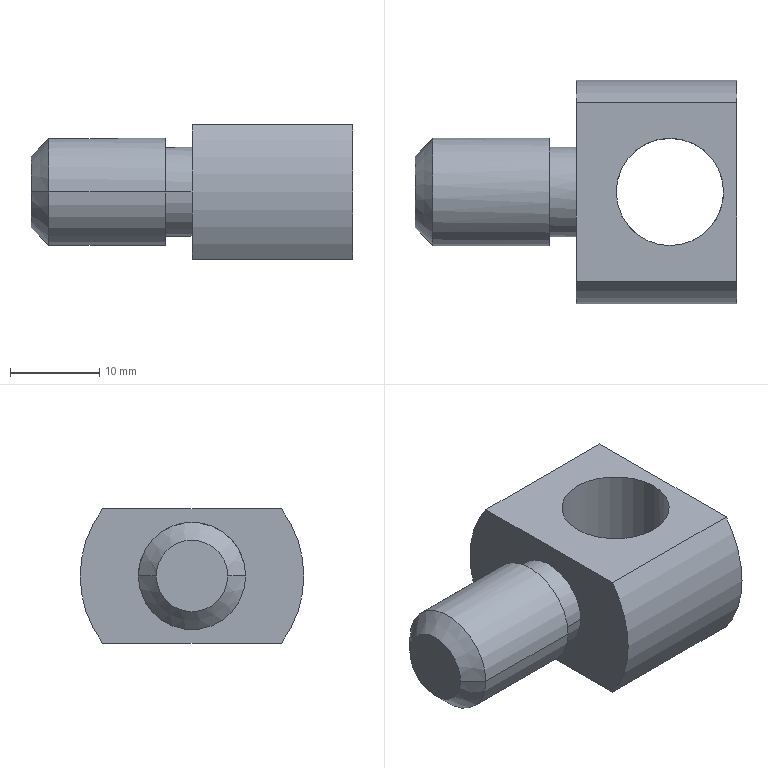Part | STEP file | Positioning_id2194_x_t | 1 solid | 16 faces | box 36 x 25 x 15 mm | volume 6488 mm3 | cylinder 8 | plane 6 | cone 2 | commonest cylinder face diameters 12 x4 10 x2 25 x2
STEP:
#1=CARTESIAN_POINT('',(0.,0.,0.));
#2=DIRECTION('',(0.,0.,1.));
#3=DIRECTION('',(1.,0.,0.));
#4=AXIS2_PLACEMENT_3D('',#1,#2,#3);
#5=CARTESIAN_POINT('',(-1029.002,410.,41.));
#6=VERTEX_POINT('',#5);
#7=CARTESIAN_POINT('',(-1031.002,412.,41.));
#8=VERTEX_POINT('',#7);
#9=CARTESIAN_POINT('',(-1031.002,412.,41.));
#10=DIRECTION('',(-0.7071,0.7071,0.));
#11=VECTOR('',#10,1.);
#12=LINE('',#9,#11);
#13=CARTESIAN_POINT('',(-1029.002,416.,41.));
#14=DIRECTION('',(1.,0.,0.));
#15=DIRECTION('',(0.,-1.,0.));
#16=AXIS2_PLACEMENT_3D('',#13,#14,#15);
#17=CONICAL_SURFACE('',#16,6.,0.7854);
#18=CARTESIAN_POINT('',(0.,-2.));
#19=DIRECTION('',(0.,-1.));
#20=VECTOR('',#19,1.);
#21=LINE('',#18,#20);
#22=(GEOMETRIC_REPRESENTATION_CONTEXT(2)PARAMETRIC_REPRESENTATION_CONTEXT()REPRESENTATION_CONTEXT('',''));
#23=DEFINITIONAL_REPRESENTATION('',(#21),#22);
#24=PCURVE('',#17,#23);
#25=CARTESIAN_POINT('',(-1029.002,416.,41.));
#26=DIRECTION('',(1.,0.,0.));
#27=DIRECTION('',(0.,-1.,0.));
#28=AXIS2_PLACEMENT_3D('',#25,#26,#27);
#29=CONICAL_SURFACE('',#28,6.,0.7854);
#30=CARTESIAN_POINT('',(6.283,-2.));
#31=DIRECTION('',(0.,-1.));
#32=VECTOR('',#31,1.);
#33=LINE('',#30,#32);
#34=(GEOMETRIC_REPRESENTATION_CONTEXT(2)PARAMETRIC_REPRESENTATION_CONTEXT()REPRESENTATION_CONTEXT('',''));
#35=DEFINITIONAL_REPRESENTATION('',(#33),#34);
#36=PCURVE('',#29,#35);
#37=SURFACE_CURVE('',#12,(#24,#36),.PCURVE_S1.);
#38=EDGE_CURVE('',#6,#8,#37,.T.);
#39=ORIENTED_EDGE('',*,*,#38,.T.);
#40=CARTESIAN_POINT('',(-1031.002,420.,41.));
#41=VERTEX_POINT('',#40);
#42=CARTESIAN_POINT('',(-1031.002,416.,41.));
#43=DIRECTION('',(-1.,0.,0.));
#44=DIRECTION('',(0.,1.,0.));
#45=AXIS2_PLACEMENT_3D('',#42,#43,#44);
#46=CIRCLE('',#45,4.);
#47=CARTESIAN_POINT('',(3.142,-2.));
#48=DIRECTION('',(-1.,0.));
#49=VECTOR('',#48,1.);
#50=LINE('',#47,#49);
#51=(GEOMETRIC_REPRESENTATION_CONTEXT(2)PARAMETRIC_REPRESENTATION_CONTEXT()REPRESENTATION_CONTEXT('',''));
#52=DEFINITIONAL_REPRESENTATION('',(#50),#51);
#53=PCURVE('',#17,#52);
#54=CARTESIAN_POINT('',(-1031.002,416.,41.));
#55=DIRECTION('',(-1.,0.,0.));
#56=DIRECTION('',(0.,1.,0.));
#57=AXIS2_PLACEMENT_3D('',#54,#55,#56);
#58=PLANE('',#57);
#59=CARTESIAN_POINT('',(0.,0.));
#60=DIRECTION('',(1.,0.));
#61=AXIS2_PLACEMENT_2D('',#59,#60);
#62=CIRCLE('',#61,4.);
#63=(GEOMETRIC_REPRESENTATION_CONTEXT(2)PARAMETRIC_REPRESENTATION_CONTEXT()REPRESENTATION_CONTEXT('',''));
#64=DEFINITIONAL_REPRESENTATION('',(#62),#63);
#65=PCURVE('',#58,#64);
#66=SURFACE_CURVE('',#46,(#53,#65),.PCURVE_S1.);
#67=EDGE_CURVE('',#41,#8,#66,.T.);
#68=ORIENTED_EDGE('',*,*,#67,.F.);
#69=CARTESIAN_POINT('',(-1029.002,422.,41.));
#70=VERTEX_POINT('',#69);
#71=CARTESIAN_POINT('',(-1031.002,420.,41.));
#72=DIRECTION('',(0.7071,0.7071,0.));
#73=VECTOR('',#72,1.);
#74=LINE('',#71,#73);
#75=CARTESIAN_POINT('',(3.142,-2.));
#76=DIRECTION('',(0.,1.));
#77=VECTOR('',#76,1.);
#78=LINE('',#75,#77);
#79=(GEOMETRIC_REPRESENTATION_CONTEXT(2)PARAMETRIC_REPRESENTATION_CONTEXT()REPRESENTATION_CONTEXT('',''));
#80=DEFINITIONAL_REPRESENTATION('',(#78),#79);
#81=PCURVE('',#17,#80);
#82=CARTESIAN_POINT('',(3.142,-2.));
#83=DIRECTION('',(0.,1.));
#84=VECTOR('',#83,1.);
#85=LINE('',#82,#84);
#86=(GEOMETRIC_REPRESENTATION_CONTEXT(2)PARAMETRIC_REPRESENTATION_CONTEXT()REPRESENTATION_CONTEXT('',''));
#87=DEFINITIONAL_REPRESENTATION('',(#85),#86);
#88=PCURVE('',#29,#87);
#89=SURFACE_CURVE('',#74,(#81,#88),.PCURVE_S1.);
#90=EDGE_CURVE('',#41,#70,#89,.T.);
#91=ORIENTED_EDGE('',*,*,#90,.T.);
#92=CARTESIAN_POINT('',(-1029.002,416.,41.));
#93=DIRECTION('',(1.,0.,0.));
#94=DIRECTION('',(0.,-1.,0.));
#95=AXIS2_PLACEMENT_3D('',#92,#93,#94);
#96=CIRCLE('',#95,6.);
#97=CARTESIAN_POINT('',(0.,0.));
#98=DIRECTION('',(1.,0.));
#99=VECTOR('',#98,1.);
#100=LINE('',#97,#99);
#101=(GEOMETRIC_REPRESENTATION_CONTEXT(2)PARAMETRIC_REPRESENTATION_CONTEXT()REPRESENTATION_CONTEXT('',''));
#102=DEFINITIONAL_REPRESENTATION('',(#100),#101);
#103=PCURVE('',#17,#102);
#104=CARTESIAN_POINT('',(-1016.002,416.,41.));
#105=DIRECTION('',(1.,0.,0.));
#106=DIRECTION('',(0.,1.,0.));
#107=AXIS2_PLACEMENT_3D('',#104,#105,#106);
#108=CYLINDRICAL_SURFACE('',#107,6.);
#109=CARTESIAN_POINT('',(3.142,-13.));
#110=DIRECTION('',(1.,0.));
#111=VECTOR('',#110,1.);
#112=LINE('',#109,#111);
#113=(GEOMETRIC_REPRESENTATION_CONTEXT(2)PARAMETRIC_REPRESENTATION_CONTEXT()REPRESENTATION_CONTEXT('',''));
#114=DEFINITIONAL_REPRESENTATION('',(#112),#113);
#115=PCURVE('',#108,#114);
#116=SURFACE_CURVE('',#96,(#103,#115),.PCURVE_S1.);
#117=EDGE_CURVE('',#6,#70,#116,.T.);
#118=ORIENTED_EDGE('',*,*,#117,.F.);
#119=EDGE_LOOP('',(#39,#68,#91,#118));
#120=FACE_BOUND('',#119,.T.);
#121=ADVANCED_FACE('',(#120),#17,.T.);
#122=CARTESIAN_POINT('',(-1016.002,422.,41.));
#123=VERTEX_POINT('',#122);
#124=CARTESIAN_POINT('',(-1016.002,422.,41.));
#125=DIRECTION('',(1.,0.,0.));
#126=VECTOR('',#125,1.);
#127=LINE('',#124,#126);
#128=CARTESIAN_POINT('',(6.283,0.));
#129=DIRECTION('',(0.,1.));
#130=VECTOR('',#129,1.);
#131=LINE('',#128,#130);
#132=(GEOMETRIC_REPRESENTATION_CONTEXT(2)PARAMETRIC_REPRESENTATION_CONTEXT()REPRESENTATION_CONTEXT('',''));
#133=DEFINITIONAL_REPRESENTATION('',(#131),#132);
#134=PCURVE('',#108,#133);
#135=CARTESIAN_POINT('',(-1016.002,416.,41.));
#136=DIRECTION('',(1.,0.,0.));
#137=DIRECTION('',(0.,1.,0.));
#138=AXIS2_PLACEMENT_3D('',#135,#136,#137);
#139=CYLINDRICAL_SURFACE('',#138,6.);
#140=CARTESIAN_POINT('',(0.,0.));
#141=DIRECTION('',(0.,1.));
#142=VECTOR('',#141,1.);
#143=LINE('',#140,#142);
#144=(GEOMETRIC_REPRESENTATION_CONTEXT(2)PARAMETRIC_REPRESENTATION_CONTEXT()REPRESENTATION_CONTEXT('',''));
#145=DEFINITIONAL_REPRESENTATION('',(#143),#144);
#146=PCURVE('',#139,#145);
#147=SURFACE_CURVE('',#127,(#134,#146),.PCURVE_S1.);
#148=EDGE_CURVE('',#70,#123,#147,.T.);
#149=ORIENTED_EDGE('',*,*,#148,.T.);
#150=CARTESIAN_POINT('',(-1016.002,410.,41.));
#151=VERTEX_POINT('',#150);
#152=CARTESIAN_POINT('',(-1016.002,416.,41.));
#153=DIRECTION('',(-1.,0.,0.));
#154=DIRECTION('',(0.,1.,0.));
#155=AXIS2_PLACEMENT_3D('',#152,#153,#154);
#156=CIRCLE('',#155,6.);
#157=CARTESIAN_POINT('',(6.283,0.));
#158=DIRECTION('',(-1.,0.));
#159=VECTOR('',#158,1.);
#160=LINE('',#157,#159);
#161=(GEOMETRIC_REPRESENTATION_CONTEXT(2)PARAMETRIC_REPRESENTATION_CONTEXT()REPRESENTATION_CONTEXT('',''));
#162=DEFINITIONAL_REPRESENTATION('',(#160),#161);
#163=PCURVE('',#108,#162);
#164=CARTESIAN_POINT('',(-1016.002,416.,41.));
#165=DIRECTION('',(1.,0.,0.));
#166=DIRECTION('',(0.,-1.,0.));
#167=AXIS2_PLACEMENT_3D('',#164,#165,#166);
#168=PLANE('',#167);
#169=CARTESIAN_POINT('',(-6.,0.));
#170=CARTESIAN_POINT('',(-6.,10.392));
#171=CARTESIAN_POINT('',(3.,5.196));
#172=CARTESIAN_POINT('',(12.,0.));
#173=CARTESIAN_POINT('',(3.,-5.196));
#174=CARTESIAN_POINT('',(-6.,-10.392));
#175=CARTESIAN_POINT('',(-6.,0.));
#176=(BOUNDED_CURVE()B_SPLINE_CURVE(2,(#169,#170,#171,#172,#173,#174,#175),.UNSPECIFIED.,.T.,.F.)B_SPLINE_CURVE_WITH_KNOTS((1,2,2,2,2,1),(-2.094,0.,2.094,4.189,6.283,8.378),.UNSPECIFIED.)CURVE()GEOMETRIC_REPRESENTATION_ITEM()RATIONAL_B_SPLINE_CURVE((1.,0.5,1.,0.5,1.,0.5,1.))REPRESENTATION_ITEM(''));
#177=(GEOMETRIC_REPRESENTATION_CONTEXT(2)PARAMETRIC_REPRESENTATION_CONTEXT()REPRESENTATION_CONTEXT('',''));
#178=DEFINITIONAL_REPRESENTATION('',(#176),#177);
#179=PCURVE('',#168,#178);
#180=SURFACE_CURVE('',#156,(#163,#179),.PCURVE_S1.);
#181=EDGE_CURVE('',#123,#151,#180,.T.);
#182=ORIENTED_EDGE('',*,*,#181,.T.);
#183=CARTESIAN_POINT('',(-1016.002,410.,41.));
#184=DIRECTION('',(-1.,0.,0.));
#185=VECTOR('',#184,1.);
#186=LINE('',#183,#185);
#187=CARTESIAN_POINT('',(3.142,0.));
#188=DIRECTION('',(0.,-1.));
#189=VECTOR('',#188,1.);
#190=LINE('',#187,#189);
#191=(GEOMETRIC_REPRESENTATION_CONTEXT(2)PARAMETRIC_REPRESENTATION_CONTEXT()REPRESENTATION_CONTEXT('',''));
#192=DEFINITIONAL_REPRESENTATION('',(#190),#191);
#193=PCURVE('',#108,#192);
#194=CARTESIAN_POINT('',(3.142,0.));
#195=DIRECTION('',(0.,-1.));
#196=VECTOR('',#195,1.);
#197=LINE('',#194,#196);
#198=(GEOMETRIC_REPRESENTATION_CONTEXT(2)PARAMETRIC_REPRESENTATION_CONTEXT()REPRESENTATION_CONTEXT('',''));
#199=DEFINITIONAL_REPRESENTATION('',(#197),#198);
#200=PCURVE('',#139,#199);
#201=SURFACE_CURVE('',#186,(#193,#200),.PCURVE_S1.);
#202=EDGE_CURVE('',#151,#6,#201,.T.);
#203=ORIENTED_EDGE('',*,*,#202,.T.);
#204=ORIENTED_EDGE('',*,*,#117,.T.);
#205=EDGE_LOOP('',(#149,#182,#203,#204));
#206=FACE_BOUND('',#205,.T.);
#207=ADVANCED_FACE('',(#206),#108,.T.);
#208=CARTESIAN_POINT('',(-1016.002,411.,41.));
#209=VERTEX_POINT('',#208);
#210=CARTESIAN_POINT('',(-1016.002,421.,41.));
#211=VERTEX_POINT('',#210);
#212=CARTESIAN_POINT('',(-1016.002,416.,41.));
#213=DIRECTION('',(-1.,0.,0.));
#214=DIRECTION('',(0.,-1.,0.));
#215=AXIS2_PLACEMENT_3D('',#212,#213,#214);
#216=CIRCLE('',#215,5.);
#217=CARTESIAN_POINT('',(5.,0.));
#218=CARTESIAN_POINT('',(5.,-8.66));
#219=CARTESIAN_POINT('',(-2.5,-4.33));
#220=CARTESIAN_POINT('',(-10.,0.));
#221=CARTESIAN_POINT('',(-2.5,4.33));
#222=CARTESIAN_POINT('',(5.,8.66));
#223=CARTESIAN_POINT('',(5.,0.));
#224=(BOUNDED_CURVE()B_SPLINE_CURVE(2,(#217,#218,#219,#220,#221,#222,#223),.UNSPECIFIED.,.T.,.F.)B_SPLINE_CURVE_WITH_KNOTS((1,2,2,2,2,1),(-2.094,0.,2.094,4.189,6.283,8.378),.UNSPECIFIED.)CURVE()GEOMETRIC_REPRESENTATION_ITEM()RATIONAL_B_SPLINE_CURVE((1.,0.5,1.,0.5,1.,0.5,1.))REPRESENTATION_ITEM(''));
#225=(GEOMETRIC_REPRESENTATION_CONTEXT(2)PARAMETRIC_REPRESENTATION_CONTEXT()REPRESENTATION_CONTEXT('',''));
#226=DEFINITIONAL_REPRESENTATION('',(#224),#225);
#227=PCURVE('',#168,#226);
#228=CARTESIAN_POINT('',(-1013.002,416.,41.));
#229=DIRECTION('',(1.,0.,0.));
#230=DIRECTION('',(0.,1.,0.));
#231=AXIS2_PLACEMENT_3D('',#228,#229,#230);
#232=CYLINDRICAL_SURFACE('',#231,5.);
#233=CARTESIAN_POINT('',(3.142,-3.));
#234=DIRECTION('',(-1.,0.));
#235=VECTOR('',#234,1.);
#236=LINE('',#233,#235);
#237=(GEOMETRIC_REPRESENTATION_CONTEXT(2)PARAMETRIC_REPRESENTATION_CONTEXT()REPRESENTATION_CONTEXT('',''));
#238=DEFINITIONAL_REPRESENTATION('',(#236),#237);
#239=PCURVE('',#232,#238);
#240=SURFACE_CURVE('',#216,(#227,#239),.PCURVE_S1.);
#241=EDGE_CURVE('',#209,#211,#240,.T.);
#242=ORIENTED_EDGE('',*,*,#241,.T.);
#243=CARTESIAN_POINT('',(-1016.002,416.,41.));
#244=DIRECTION('',(-1.,0.,0.));
#245=DIRECTION('',(0.,1.,0.));
#246=AXIS2_PLACEMENT_3D('',#243,#244,#245);
#247=CIRCLE('',#246,5.);
#248=CARTESIAN_POINT('',(-5.,0.));
#249=CARTESIAN_POINT('',(-5.,8.66));
#250=CARTESIAN_POINT('',(2.5,4.33));
#251=CARTESIAN_POINT('',(10.,0.));
#252=CARTESIAN_POINT('',(2.5,-4.33));
#253=CARTESIAN_POINT('',(-5.,-8.66));
#254=CARTESIAN_POINT('',(-5.,0.));
#255=(BOUNDED_CURVE()B_SPLINE_CURVE(2,(#248,#249,#250,#251,#252,#253,#254),.UNSPECIFIED.,.T.,.F.)B_SPLINE_CURVE_WITH_KNOTS((1,2,2,2,2,1),(-2.094,0.,2.094,4.189,6.283,8.378),.UNSPECIFIED.)CURVE()GEOMETRIC_REPRESENTATION_ITEM()RATIONAL_B_SPLINE_CURVE((1.,0.5,1.,0.5,1.,0.5,1.))REPRESENTATION_ITEM(''));
#256=(GEOMETRIC_REPRESENTATION_CONTEXT(2)PARAMETRIC_REPRESENTATION_CONTEXT()REPRESENTATION_CONTEXT('',''));
#257=DEFINITIONAL_REPRESENTATION('',(#255),#256);
#258=PCURVE('',#168,#257);
#259=CARTESIAN_POINT('',(-1013.002,416.,41.));
#260=DIRECTION('',(1.,0.,0.));
#261=DIRECTION('',(0.,1.,0.));
#262=AXIS2_PLACEMENT_3D('',#259,#260,#261);
#263=CYLINDRICAL_SURFACE('',#262,5.);
#264=CARTESIAN_POINT('',(6.283,-3.));
#265=DIRECTION('',(-1.,0.));
#266=VECTOR('',#265,1.);
#267=LINE('',#264,#266);
#268=(GEOMETRIC_REPRESENTATION_CONTEXT(2)PARAMETRIC_REPRESENTATION_CONTEXT()REPRESENTATION_CONTEXT('',''));
#269=DEFINITIONAL_REPRESENTATION('',(#267),#268);
#270=PCURVE('',#263,#269);
#271=SURFACE_CURVE('',#247,(#258,#270),.PCURVE_S1.);
#272=EDGE_CURVE('',#211,#209,#271,.T.);
#273=ORIENTED_EDGE('',*,*,#272,.T.);
#274=EDGE_LOOP('',(#242,#273));
#275=FACE_BOUND('',#274,.T.);
#276=CARTESIAN_POINT('',(-1016.002,410.,41.));
#277=CARTESIAN_POINT('',(-1016.002,410.,47.));
#278=CARTESIAN_POINT('',(-1016.002,416.,50.));
#279=CARTESIAN_POINT('',(-1016.002,422.,47.));
#280=CARTESIAN_POINT('',(-1016.002,422.,41.));
#281=(BOUNDED_CURVE()B_SPLINE_CURVE(4,(#276,#277,#278,#279,#280),.UNSPECIFIED.,.F.,.F.)B_SPLINE_CURVE_WITH_KNOTS((5,5),(0.,1.),.PIECEWISE_BEZIER_KNOTS.)CURVE()GEOMETRIC_REPRESENTATION_ITEM()RATIONAL_B_SPLINE_CURVE((1.,0.7071,0.6667,0.7071,1.))REPRESENTATION_ITEM(''));
#282=CARTESIAN_POINT('',(6.,0.));
#283=CARTESIAN_POINT('',(6.,-6.));
#284=CARTESIAN_POINT('',(0.,-9.));
#285=CARTESIAN_POINT('',(-6.,-6.));
#286=CARTESIAN_POINT('',(-6.,0.));
#287=(BOUNDED_CURVE()B_SPLINE_CURVE(4,(#282,#283,#284,#285,#286),.UNSPECIFIED.,.F.,.F.)B_SPLINE_CURVE_WITH_KNOTS((5,5),(0.,1.),.PIECEWISE_BEZIER_KNOTS.)CURVE()GEOMETRIC_REPRESENTATION_ITEM()RATIONAL_B_SPLINE_CURVE((1.,0.7071,0.6667,0.7071,1.))REPRESENTATION_ITEM(''));
#288=(GEOMETRIC_REPRESENTATION_CONTEXT(2)PARAMETRIC_REPRESENTATION_CONTEXT()REPRESENTATION_CONTEXT('',''));
#289=DEFINITIONAL_REPRESENTATION('',(#287),#288);
#290=PCURVE('',#168,#289);
#291=CARTESIAN_POINT('',(3.142,0.));
#292=CARTESIAN_POINT('',(3.099,0.));
#293=CARTESIAN_POINT('',(3.012,0.));
#294=CARTESIAN_POINT('',(2.878,0.));
#295=CARTESIAN_POINT('',(2.742,0.));
#296=CARTESIAN_POINT('',(2.602,0.));
#297=CARTESIAN_POINT('',(2.46,0.));
#298=CARTESIAN_POINT('',(2.316,0.));
#299=CARTESIAN_POINT('',(2.169,0.));
#300=CARTESIAN_POINT('',(2.021,0.));
#301=CARTESIAN_POINT('',(1.872,0.));
#302=CARTESIAN_POINT('',(1.721,0.));
#303=CARTESIAN_POINT('',(1.571,0.));
#304=CARTESIAN_POINT('',(1.42,0.));
#305=CARTESIAN_POINT('',(1.27,0.));
#306=CARTESIAN_POINT('',(1.121,0.));
#307=CARTESIAN_POINT('',(0.9725,0.));
#308=CARTESIAN_POINT('',(0.8261,0.));
#309=CARTESIAN_POINT('',(0.6816,0.));
#310=CARTESIAN_POINT('',(0.5394,0.));
#311=CARTESIAN_POINT('',(0.3999,0.));
#312=CARTESIAN_POINT('',(0.2633,0.));
#313=CARTESIAN_POINT('',(0.1297,0.));
#314=CARTESIAN_POINT('',(0.04285,0.));
#315=CARTESIAN_POINT('',(0.,0.));
#316=B_SPLINE_CURVE_WITH_KNOTS('',3,(#291,#292,#293,#294,#295,#296,#297,#298,#299,#300,#301,#302,#303,#304,#305,#306,#307,#308,#309,#310,#311,#312,#313,#314,#315),.UNSPECIFIED.,.F.,.F.,(4,1,1,1,1,1,1,1,1,1,1,1,1,1,1,1,1,1,1,1,1,1,4),(0.,0.04545,0.09091,0.1364,0.1818,0.2273,0.2727,0.3182,0.3636,0.4091,0.4545,0.5,0.5455,0.5909,0.6364,0.6818,0.7273,0.7727,0.8182,0.8636,0.9091,0.9545,1.),.QUASI_UNIFORM_KNOTS.);
#317=(GEOMETRIC_REPRESENTATION_CONTEXT(2)PARAMETRIC_REPRESENTATION_CONTEXT()REPRESENTATION_CONTEXT('',''));
#318=DEFINITIONAL_REPRESENTATION('',(#316),#317);
#319=PCURVE('',#139,#318);
#320=SURFACE_CURVE('',#281,(#290,#319),.PCURVE_S1.);
#321=EDGE_CURVE('',#151,#123,#320,.T.);
#322=ORIENTED_EDGE('',*,*,#321,.F.);
#323=ORIENTED_EDGE('',*,*,#181,.F.);
#324=EDGE_LOOP('',(#322,#323));
#325=FACE_BOUND('',#324,.T.);
#326=ADVANCED_FACE('',(#275,#325),#168,.T.);
#327=ORIENTED_EDGE('',*,*,#67,.T.);
#328=CARTESIAN_POINT('',(-1031.002,412.,41.));
#329=CARTESIAN_POINT('',(-1031.002,412.,45.));
#330=CARTESIAN_POINT('',(-1031.002,416.,47.));
#331=CARTESIAN_POINT('',(-1031.002,420.,45.));
#332=CARTESIAN_POINT('',(-1031.002,420.,41.));
#333=(BOUNDED_CURVE()B_SPLINE_CURVE(4,(#328,#329,#330,#331,#332),.UNSPECIFIED.,.F.,.F.)B_SPLINE_CURVE_WITH_KNOTS((5,5),(0.,1.),.PIECEWISE_BEZIER_KNOTS.)CURVE()GEOMETRIC_REPRESENTATION_ITEM()RATIONAL_B_SPLINE_CURVE((1.,0.7071,0.6667,0.7071,1.))REPRESENTATION_ITEM(''));
#334=CARTESIAN_POINT('',(-4.,0.));
#335=CARTESIAN_POINT('',(-4.,-4.));
#336=CARTESIAN_POINT('',(0.,-6.));
#337=CARTESIAN_POINT('',(4.,-4.));
#338=CARTESIAN_POINT('',(4.,0.));
#339=(BOUNDED_CURVE()B_SPLINE_CURVE(4,(#334,#335,#336,#337,#338),.UNSPECIFIED.,.F.,.F.)B_SPLINE_CURVE_WITH_KNOTS((5,5),(0.,1.),.PIECEWISE_BEZIER_KNOTS.)CURVE()GEOMETRIC_REPRESENTATION_ITEM()RATIONAL_B_SPLINE_CURVE((1.,0.7071,0.6667,0.7071,1.))REPRESENTATION_ITEM(''));
#340=(GEOMETRIC_REPRESENTATION_CONTEXT(2)PARAMETRIC_REPRESENTATION_CONTEXT()REPRESENTATION_CONTEXT('',''));
#341=DEFINITIONAL_REPRESENTATION('',(#339),#340);
#342=PCURVE('',#58,#341);
#343=CARTESIAN_POINT('',(6.283,-2.));
#344=CARTESIAN_POINT('',(6.24,-2.));
#345=CARTESIAN_POINT('',(6.153,-2.));
#346=CARTESIAN_POINT('',(6.02,-2.));
#347=CARTESIAN_POINT('',(5.883,-2.));
#348=CARTESIAN_POINT('',(5.744,-2.));
#349=CARTESIAN_POINT('',(5.602,-2.));
#350=CARTESIAN_POINT('',(5.457,-2.));
#351=CARTESIAN_POINT('',(5.311,-2.));
#352=CARTESIAN_POINT('',(5.163,-2.));
#353=CARTESIAN_POINT('',(5.013,-2.));
#354=CARTESIAN_POINT('',(4.863,-2.));
#355=CARTESIAN_POINT('',(4.712,-2.));
#356=CARTESIAN_POINT('',(4.562,-2.));
#357=CARTESIAN_POINT('',(4.412,-2.));
#358=CARTESIAN_POINT('',(4.262,-2.));
#359=CARTESIAN_POINT('',(4.114,-2.));
#360=CARTESIAN_POINT('',(3.968,-2.));
#361=CARTESIAN_POINT('',(3.823,-2.));
#362=CARTESIAN_POINT('',(3.681,-2.));
#363=CARTESIAN_POINT('',(3.542,-2.));
#364=CARTESIAN_POINT('',(3.405,-2.));
#365=CARTESIAN_POINT('',(3.271,-2.));
#366=CARTESIAN_POINT('',(3.184,-2.));
#367=CARTESIAN_POINT('',(3.142,-2.));
#368=B_SPLINE_CURVE_WITH_KNOTS('',3,(#343,#344,#345,#346,#347,#348,#349,#350,#351,#352,#353,#354,#355,#356,#357,#358,#359,#360,#361,#362,#363,#364,#365,#366,#367),.UNSPECIFIED.,.F.,.F.,(4,1,1,1,1,1,1,1,1,1,1,1,1,1,1,1,1,1,1,1,1,1,4),(0.,0.04545,0.09091,0.1364,0.1818,0.2273,0.2727,0.3182,0.3636,0.4091,0.4545,0.5,0.5455,0.5909,0.6364,0.6818,0.7273,0.7727,0.8182,0.8636,0.9091,0.9545,1.),.QUASI_UNIFORM_KNOTS.);
#369=(GEOMETRIC_REPRESENTATION_CONTEXT(2)PARAMETRIC_REPRESENTATION_CONTEXT()REPRESENTATION_CONTEXT('',''));
#370=DEFINITIONAL_REPRESENTATION('',(#368),#369);
#371=PCURVE('',#29,#370);
#372=SURFACE_CURVE('',#333,(#342,#371),.PCURVE_S1.);
#373=EDGE_CURVE('',#8,#41,#372,.T.);
#374=ORIENTED_EDGE('',*,*,#373,.T.);
#375=EDGE_LOOP('',(#327,#374));
#376=FACE_BOUND('',#375,.T.);
#377=ADVANCED_FACE('',(#376),#58,.T.);
#378=CARTESIAN_POINT('',(-1013.002,421.,41.));
#379=VERTEX_POINT('',#378);
#380=CARTESIAN_POINT('',(-1013.002,421.,41.));
#381=DIRECTION('',(1.,0.,0.));
#382=VECTOR('',#381,1.);
#383=LINE('',#380,#382);
#384=CARTESIAN_POINT('',(6.283,0.));
#385=DIRECTION('',(0.,1.));
#386=VECTOR('',#385,1.);
#387=LINE('',#384,#386);
#388=(GEOMETRIC_REPRESENTATION_CONTEXT(2)PARAMETRIC_REPRESENTATION_CONTEXT()REPRESENTATION_CONTEXT('',''));
#389=DEFINITIONAL_REPRESENTATION('',(#387),#388);
#390=PCURVE('',#263,#389);
#391=CARTESIAN_POINT('',(0.,0.));
#392=DIRECTION('',(0.,1.));
#393=VECTOR('',#392,1.);
#394=LINE('',#391,#393);
#395=(GEOMETRIC_REPRESENTATION_CONTEXT(2)PARAMETRIC_REPRESENTATION_CONTEXT()REPRESENTATION_CONTEXT('',''));
#396=DEFINITIONAL_REPRESENTATION('',(#394),#395);
#397=PCURVE('',#232,#396);
#398=SURFACE_CURVE('',#383,(#390,#397),.PCURVE_S1.);
#399=EDGE_CURVE('',#211,#379,#398,.T.);
#400=ORIENTED_EDGE('',*,*,#399,.T.);
#401=CARTESIAN_POINT('',(-1013.002,411.,41.));
#402=VERTEX_POINT('',#401);
#403=CARTESIAN_POINT('',(-1013.002,416.,41.));
#404=DIRECTION('',(-1.,0.,0.));
#405=DIRECTION('',(0.,1.,0.));
#406=AXIS2_PLACEMENT_3D('',#403,#404,#405);
#407=CIRCLE('',#406,5.);
#408=CARTESIAN_POINT('',(6.283,0.));
#409=DIRECTION('',(-1.,0.));
#410=VECTOR('',#409,1.);
#411=LINE('',#408,#410);
#412=(GEOMETRIC_REPRESENTATION_CONTEXT(2)PARAMETRIC_REPRESENTATION_CONTEXT()REPRESENTATION_CONTEXT('',''));
#413=DEFINITIONAL_REPRESENTATION('',(#411),#412);
#414=PCURVE('',#263,#413);
#415=CARTESIAN_POINT('',(-1013.002,416.,41.));
#416=DIRECTION('',(-1.,0.,0.));
#417=DIRECTION('',(0.,0.,-1.));
#418=AXIS2_PLACEMENT_3D('',#415,#416,#417);
#419=PLANE('',#418);
#420=CARTESIAN_POINT('',(0.,0.));
#421=DIRECTION('',(0.,-1.));
#422=AXIS2_PLACEMENT_2D('',#420,#421);
#423=CIRCLE('',#422,5.);
#424=(GEOMETRIC_REPRESENTATION_CONTEXT(2)PARAMETRIC_REPRESENTATION_CONTEXT()REPRESENTATION_CONTEXT('',''));
#425=DEFINITIONAL_REPRESENTATION('',(#423),#424);
#426=PCURVE('',#419,#425);
#427=SURFACE_CURVE('',#407,(#414,#426),.PCURVE_S1.);
#428=EDGE_CURVE('',#379,#402,#427,.T.);
#429=ORIENTED_EDGE('',*,*,#428,.T.);
#430=CARTESIAN_POINT('',(-1013.002,411.,41.));
#431=DIRECTION('',(-1.,0.,0.));
#432=VECTOR('',#431,1.);
#433=LINE('',#430,#432);
#434=CARTESIAN_POINT('',(3.142,0.));
#435=DIRECTION('',(0.,-1.));
#436=VECTOR('',#435,1.);
#437=LINE('',#434,#436);
#438=(GEOMETRIC_REPRESENTATION_CONTEXT(2)PARAMETRIC_REPRESENTATION_CONTEXT()REPRESENTATION_CONTEXT('',''));
#439=DEFINITIONAL_REPRESENTATION('',(#437),#438);
#440=PCURVE('',#263,#439);
#441=CARTESIAN_POINT('',(3.142,0.));
#442=DIRECTION('',(0.,-1.));
#443=VECTOR('',#442,1.);
#444=LINE('',#441,#443);
#445=(GEOMETRIC_REPRESENTATION_CONTEXT(2)PARAMETRIC_REPRESENTATION_CONTEXT()REPRESENTATION_CONTEXT('',''));
#446=DEFINITIONAL_REPRESENTATION('',(#444),#445);
#447=PCURVE('',#232,#446);
#448=SURFACE_CURVE('',#433,(#440,#447),.PCURVE_S1.);
#449=EDGE_CURVE('',#402,#209,#448,.T.);
#450=ORIENTED_EDGE('',*,*,#449,.T.);
#451=ORIENTED_EDGE('',*,*,#272,.F.);
#452=EDGE_LOOP('',(#400,#429,#450,#451));
#453=FACE_BOUND('',#452,.T.);
#454=ADVANCED_FACE('',(#453),#263,.T.);
#455=CARTESIAN_POINT('',(-1002.502,422.,33.5));
#456=VERTEX_POINT('',#455);
#457=CARTESIAN_POINT('',(-996.502,416.,33.5));
#458=VERTEX_POINT('',#457);
#459=CARTESIAN_POINT('',(-1002.502,416.,33.5));
#460=DIRECTION('',(0.,0.,-1.));
#461=DIRECTION('',(0.,-1.,0.));
#462=AXIS2_PLACEMENT_3D('',#459,#460,#461);
#463=CIRCLE('',#462,6.);
#464=CARTESIAN_POINT('',(-1002.502,416.,47.));
#465=DIRECTION('',(0.,0.,1.));
#466=DIRECTION('',(1.,0.,0.));
#467=AXIS2_PLACEMENT_3D('',#464,#465,#466);
#468=CYLINDRICAL_SURFACE('',#467,6.);
#469=CARTESIAN_POINT('',(4.712,-13.5));
#470=DIRECTION('',(-1.,0.));
#471=VECTOR('',#470,1.);
#472=LINE('',#469,#471);
#473=(GEOMETRIC_REPRESENTATION_CONTEXT(2)PARAMETRIC_REPRESENTATION_CONTEXT()REPRESENTATION_CONTEXT('',''));
#474=DEFINITIONAL_REPRESENTATION('',(#472),#473);
#475=PCURVE('',#468,#474);
#476=CARTESIAN_POINT('',(-1010.002,416.,33.5));
#477=DIRECTION('',(0.,0.,1.));
#478=DIRECTION('',(-1.,0.,0.));
#479=AXIS2_PLACEMENT_3D('',#476,#477,#478);
#480=PLANE('',#479);
#481=CARTESIAN_POINT('',(-7.5,6.));
#482=CARTESIAN_POINT('',(2.892,6.));
#483=CARTESIAN_POINT('',(-2.304,-3.));
#484=CARTESIAN_POINT('',(-7.5,-12.));
#485=CARTESIAN_POINT('',(-12.696,-3.));
#486=CARTESIAN_POINT('',(-17.892,6.));
#487=CARTESIAN_POINT('',(-7.5,6.));
#488=(BOUNDED_CURVE()B_SPLINE_CURVE(2,(#481,#482,#483,#484,#485,#486,#487),.UNSPECIFIED.,.T.,.F.)B_SPLINE_CURVE_WITH_KNOTS((1,2,2,2,2,1),(-2.094,0.,2.094,4.189,6.283,8.378),.UNSPECIFIED.)CURVE()GEOMETRIC_REPRESENTATION_ITEM()RATIONAL_B_SPLINE_CURVE((1.,0.5,1.,0.5,1.,0.5,1.))REPRESENTATION_ITEM(''));
#489=(GEOMETRIC_REPRESENTATION_CONTEXT(2)PARAMETRIC_REPRESENTATION_CONTEXT()REPRESENTATION_CONTEXT('',''));
#490=DEFINITIONAL_REPRESENTATION('',(#488),#489);
#491=PCURVE('',#480,#490);
#492=SURFACE_CURVE('',#463,(#475,#491),.PCURVE_S1.);
#493=EDGE_CURVE('',#456,#458,#492,.T.);
#494=ORIENTED_EDGE('',*,*,#493,.F.);
#495=CARTESIAN_POINT('',(-1008.502,416.,33.5));
#496=VERTEX_POINT('',#495);
#497=CARTESIAN_POINT('',(-1002.502,416.,33.5));
#498=DIRECTION('',(0.,0.,-1.));
#499=DIRECTION('',(0.,-1.,0.));
#500=AXIS2_PLACEMENT_3D('',#497,#498,#499);
#501=CIRCLE('',#500,6.);
#502=CARTESIAN_POINT('',(4.712,-13.5));
#503=DIRECTION('',(-1.,0.));
#504=VECTOR('',#503,1.);
#505=LINE('',#502,#504);
#506=(GEOMETRIC_REPRESENTATION_CONTEXT(2)PARAMETRIC_REPRESENTATION_CONTEXT()REPRESENTATION_CONTEXT('',''));
#507=DEFINITIONAL_REPRESENTATION('',(#505),#506);
#508=PCURVE('',#468,#507);
#509=CARTESIAN_POINT('',(-7.5,6.));
#510=CARTESIAN_POINT('',(2.892,6.));
#511=CARTESIAN_POINT('',(-2.304,-3.));
#512=CARTESIAN_POINT('',(-7.5,-12.));
#513=CARTESIAN_POINT('',(-12.696,-3.));
#514=CARTESIAN_POINT('',(-17.892,6.));
#515=CARTESIAN_POINT('',(-7.5,6.));
#516=(BOUNDED_CURVE()B_SPLINE_CURVE(2,(#509,#510,#511,#512,#513,#514,#515),.UNSPECIFIED.,.T.,.F.)B_SPLINE_CURVE_WITH_KNOTS((1,2,2,2,2,1),(-2.094,0.,2.094,4.189,6.283,8.378),.UNSPECIFIED.)CURVE()GEOMETRIC_REPRESENTATION_ITEM()RATIONAL_B_SPLINE_CURVE((1.,0.5,1.,0.5,1.,0.5,1.))REPRESENTATION_ITEM(''));
#517=(GEOMETRIC_REPRESENTATION_CONTEXT(2)PARAMETRIC_REPRESENTATION_CONTEXT()REPRESENTATION_CONTEXT('',''));
#518=DEFINITIONAL_REPRESENTATION('',(#516),#517);
#519=PCURVE('',#480,#518);
#520=SURFACE_CURVE('',#501,(#508,#519),.PCURVE_S1.);
#521=EDGE_CURVE('',#496,#456,#520,.T.);
#522=ORIENTED_EDGE('',*,*,#521,.F.);
#523=CARTESIAN_POINT('',(-1008.502,416.,48.5));
#524=VERTEX_POINT('',#523);
#525=CARTESIAN_POINT('',(-1008.502,416.,48.5));
#526=DIRECTION('',(0.,0.,-1.));
#527=VECTOR('',#526,1.);
#528=LINE('',#525,#527);
#529=CARTESIAN_POINT('',(3.142,1.5));
#530=DIRECTION('',(0.,-1.));
#531=VECTOR('',#530,1.);
#532=LINE('',#529,#531);
#533=(GEOMETRIC_REPRESENTATION_CONTEXT(2)PARAMETRIC_REPRESENTATION_CONTEXT()REPRESENTATION_CONTEXT('',''));
#534=DEFINITIONAL_REPRESENTATION('',(#532),#533);
#535=PCURVE('',#468,#534);
#536=CARTESIAN_POINT('',(-1002.502,416.,47.));
#537=DIRECTION('',(0.,0.,1.));
#538=DIRECTION('',(1.,0.,0.));
#539=AXIS2_PLACEMENT_3D('',#536,#537,#538);
#540=CYLINDRICAL_SURFACE('',#539,6.);
#541=CARTESIAN_POINT('',(3.142,1.5));
#542=DIRECTION('',(0.,-1.));
#543=VECTOR('',#542,1.);
#544=LINE('',#541,#543);
#545=(GEOMETRIC_REPRESENTATION_CONTEXT(2)PARAMETRIC_REPRESENTATION_CONTEXT()REPRESENTATION_CONTEXT('',''));
#546=DEFINITIONAL_REPRESENTATION('',(#544),#545);
#547=PCURVE('',#540,#546);
#548=SURFACE_CURVE('',#528,(#535,#547),.PCURVE_S1.);
#549=EDGE_CURVE('',#524,#496,#548,.T.);
#550=ORIENTED_EDGE('',*,*,#549,.F.);
#551=CARTESIAN_POINT('',(-1002.502,422.,48.5));
#552=VERTEX_POINT('',#551);
#553=CARTESIAN_POINT('',(-1002.502,416.,48.5));
#554=DIRECTION('',(0.,0.,1.));
#555=DIRECTION('',(0.,-1.,0.));
#556=AXIS2_PLACEMENT_3D('',#553,#554,#555);
#557=CIRCLE('',#556,6.);
#558=CARTESIAN_POINT('',(-1.571,1.5));
#559=DIRECTION('',(1.,0.));
#560=VECTOR('',#559,1.);
#561=LINE('',#558,#560);
#562=(GEOMETRIC_REPRESENTATION_CONTEXT(2)PARAMETRIC_REPRESENTATION_CONTEXT()REPRESENTATION_CONTEXT('',''));
#563=DEFINITIONAL_REPRESENTATION('',(#561),#562);
#564=PCURVE('',#468,#563);
#565=CARTESIAN_POINT('',(-1002.502,416.,48.5));
#566=DIRECTION('',(0.,0.,1.));
#567=DIRECTION('',(-1.,0.,0.));
#568=AXIS2_PLACEMENT_3D('',#565,#566,#567);
#569=PLANE('',#568);
#570=CARTESIAN_POINT('',(0.,0.));
#571=DIRECTION('',(0.,1.));
#572=AXIS2_PLACEMENT_2D('',#570,#571);
#573=CIRCLE('',#572,6.);
#574=(GEOMETRIC_REPRESENTATION_CONTEXT(2)PARAMETRIC_REPRESENTATION_CONTEXT()REPRESENTATION_CONTEXT('',''));
#575=DEFINITIONAL_REPRESENTATION('',(#573),#574);
#576=PCURVE('',#569,#575);
#577=SURFACE_CURVE('',#557,(#564,#576),.PCURVE_S1.);
#578=EDGE_CURVE('',#552,#524,#577,.T.);
#579=ORIENTED_EDGE('',*,*,#578,.F.);
#580=CARTESIAN_POINT('',(-996.502,416.,48.5));
#581=VERTEX_POINT('',#580);
#582=CARTESIAN_POINT('',(-1002.502,416.,48.5));
#583=DIRECTION('',(0.,0.,1.));
#584=DIRECTION('',(0.,-1.,0.));
#585=AXIS2_PLACEMENT_3D('',#582,#583,#584);
#586=CIRCLE('',#585,6.);
#587=CARTESIAN_POINT('',(-1.571,1.5));
#588=DIRECTION('',(1.,0.));
#589=VECTOR('',#588,1.);
#590=LINE('',#587,#589);
#591=(GEOMETRIC_REPRESENTATION_CONTEXT(2)PARAMETRIC_REPRESENTATION_CONTEXT()REPRESENTATION_CONTEXT('',''));
#592=DEFINITIONAL_REPRESENTATION('',(#590),#591);
#593=PCURVE('',#468,#592);
#594=CARTESIAN_POINT('',(0.,0.));
#595=DIRECTION('',(0.,1.));
#596=AXIS2_PLACEMENT_2D('',#594,#595);
#597=CIRCLE('',#596,6.);
#598=(GEOMETRIC_REPRESENTATION_CONTEXT(2)PARAMETRIC_REPRESENTATION_CONTEXT()REPRESENTATION_CONTEXT('',''));
#599=DEFINITIONAL_REPRESENTATION('',(#597),#598);
#600=PCURVE('',#569,#599);
#601=SURFACE_CURVE('',#586,(#593,#600),.PCURVE_S1.);
#602=EDGE_CURVE('',#581,#552,#601,.T.);
#603=ORIENTED_EDGE('',*,*,#602,.F.);
#604=CARTESIAN_POINT('',(-996.502,416.,48.5));
#605=DIRECTION('',(0.,0.,1.));
#606=VECTOR('',#605,1.);
#607=LINE('',#604,#606);
#608=CARTESIAN_POINT('',(0.,1.5));
#609=DIRECTION('',(0.,1.));
#610=VECTOR('',#609,1.);
#611=LINE('',#608,#610);
#612=(GEOMETRIC_REPRESENTATION_CONTEXT(2)PARAMETRIC_REPRESENTATION_CONTEXT()REPRESENTATION_CONTEXT('',''));
#613=DEFINITIONAL_REPRESENTATION('',(#611),#612);
#614=PCURVE('',#468,#613);
#615=CARTESIAN_POINT('',(6.283,1.5));
#616=DIRECTION('',(0.,1.));
#617=VECTOR('',#616,1.);
#618=LINE('',#615,#617);
#619=(GEOMETRIC_REPRESENTATION_CONTEXT(2)PARAMETRIC_REPRESENTATION_CONTEXT()REPRESENTATION_CONTEXT('',''));
#620=DEFINITIONAL_REPRESENTATION('',(#618),#619);
#621=PCURVE('',#540,#620);
#622=SURFACE_CURVE('',#607,(#614,#621),.PCURVE_S1.);
#623=EDGE_CURVE('',#458,#581,#622,.T.);
#624=ORIENTED_EDGE('',*,*,#623,.F.);
#625=EDGE_LOOP('',(#494,#522,#550,#579,#603,#624));
#626=FACE_BOUND('',#625,.F.);
#627=ADVANCED_FACE('',(#626),#468,.F.);
#628=ORIENTED_EDGE('',*,*,#521,.F.);
#629=CARTESIAN_POINT('',(-996.502,416.,33.5));
#630=CARTESIAN_POINT('',(-996.502,410.,33.5));
#631=CARTESIAN_POINT('',(-1002.502,407.,33.5));
#632=CARTESIAN_POINT('',(-1008.502,410.,33.5));
#633=CARTESIAN_POINT('',(-1008.502,416.,33.5));
#634=(BOUNDED_CURVE()B_SPLINE_CURVE(4,(#629,#630,#631,#632,#633),.UNSPECIFIED.,.F.,.F.)B_SPLINE_CURVE_WITH_KNOTS((5,5),(0.,1.),.PIECEWISE_BEZIER_KNOTS.)CURVE()GEOMETRIC_REPRESENTATION_ITEM()RATIONAL_B_SPLINE_CURVE((1.,0.7071,0.6667,0.7071,1.))REPRESENTATION_ITEM(''));
#635=CARTESIAN_POINT('',(-13.5,0.));
#636=CARTESIAN_POINT('',(-13.5,6.));
#637=CARTESIAN_POINT('',(-7.5,9.));
#638=CARTESIAN_POINT('',(-1.5,6.));
#639=CARTESIAN_POINT('',(-1.5,0.));
#640=(BOUNDED_CURVE()B_SPLINE_CURVE(4,(#635,#636,#637,#638,#639),.UNSPECIFIED.,.F.,.F.)B_SPLINE_CURVE_WITH_KNOTS((5,5),(0.,1.),.PIECEWISE_BEZIER_KNOTS.)CURVE()GEOMETRIC_REPRESENTATION_ITEM()RATIONAL_B_SPLINE_CURVE((1.,0.7071,0.6667,0.7071,1.))REPRESENTATION_ITEM(''));
#641=(GEOMETRIC_REPRESENTATION_CONTEXT(2)PARAMETRIC_REPRESENTATION_CONTEXT()REPRESENTATION_CONTEXT('',''));
#642=DEFINITIONAL_REPRESENTATION('',(#640),#641);
#643=PCURVE('',#480,#642);
#644=CARTESIAN_POINT('',(6.283,-13.5));
#645=CARTESIAN_POINT('',(6.24,-13.5));
#646=CARTESIAN_POINT('',(6.153,-13.5));
#647=CARTESIAN_POINT('',(6.02,-13.5));
#648=CARTESIAN_POINT('',(5.883,-13.5));
#649=CARTESIAN_POINT('',(5.744,-13.5));
#650=CARTESIAN_POINT('',(5.602,-13.5));
#651=CARTESIAN_POINT('',(5.457,-13.5));
#652=CARTESIAN_POINT('',(5.311,-13.5));
#653=CARTESIAN_POINT('',(5.163,-13.5));
#654=CARTESIAN_POINT('',(5.013,-13.5));
#655=CARTESIAN_POINT('',(4.863,-13.5));
#656=CARTESIAN_POINT('',(4.712,-13.5));
#657=CARTESIAN_POINT('',(4.562,-13.5));
#658=CARTESIAN_POINT('',(4.412,-13.5));
#659=CARTESIAN_POINT('',(4.262,-13.5));
#660=CARTESIAN_POINT('',(4.114,-13.5));
#661=CARTESIAN_POINT('',(3.968,-13.5));
#662=CARTESIAN_POINT('',(3.823,-13.5));
#663=CARTESIAN_POINT('',(3.681,-13.5));
#664=CARTESIAN_POINT('',(3.542,-13.5));
#665=CARTESIAN_POINT('',(3.405,-13.5));
#666=CARTESIAN_POINT('',(3.271,-13.5));
#667=CARTESIAN_POINT('',(3.184,-13.5));
#668=CARTESIAN_POINT('',(3.142,-13.5));
#669=B_SPLINE_CURVE_WITH_KNOTS('',3,(#644,#645,#646,#647,#648,#649,#650,#651,#652,#653,#654,#655,#656,#657,#658,#659,#660,#661,#662,#663,#664,#665,#666,#667,#668),.UNSPECIFIED.,.F.,.F.,(4,1,1,1,1,1,1,1,1,1,1,1,1,1,1,1,1,1,1,1,1,1,4),(0.,0.04545,0.09091,0.1364,0.1818,0.2273,0.2727,0.3182,0.3636,0.4091,0.4545,0.5,0.5455,0.5909,0.6364,0.6818,0.7273,0.7727,0.8182,0.8636,0.9091,0.9545,1.),.QUASI_UNIFORM_KNOTS.);
#670=(GEOMETRIC_REPRESENTATION_CONTEXT(2)PARAMETRIC_REPRESENTATION_CONTEXT()REPRESENTATION_CONTEXT('',''));
#671=DEFINITIONAL_REPRESENTATION('',(#669),#670);
#672=PCURVE('',#540,#671);
#673=SURFACE_CURVE('',#634,(#643,#672),.PCURVE_S1.);
#674=EDGE_CURVE('',#458,#496,#673,.T.);
#675=ORIENTED_EDGE('',*,*,#674,.F.);
#676=ORIENTED_EDGE('',*,*,#493,.F.);
#677=EDGE_LOOP('',(#628,#675,#676));
#678=FACE_BOUND('',#677,.T.);
#679=CARTESIAN_POINT('',(-995.002,406.,33.5));
#680=VERTEX_POINT('',#679);
#681=CARTESIAN_POINT('',(-995.002,426.,33.5));
#682=VERTEX_POINT('',#681);
#683=CARTESIAN_POINT('',(-995.002,406.,33.5));
#684=DIRECTION('',(0.,1.,0.));
#685=VECTOR('',#684,1.);
#686=LINE('',#683,#685);
#687=CARTESIAN_POINT('',(-15.,10.));
#688=DIRECTION('',(0.,-1.));
#689=VECTOR('',#688,1.);
#690=LINE('',#687,#689);
#691=(GEOMETRIC_REPRESENTATION_CONTEXT(2)PARAMETRIC_REPRESENTATION_CONTEXT()REPRESENTATION_CONTEXT('',''));
#692=DEFINITIONAL_REPRESENTATION('',(#690),#691);
#693=PCURVE('',#480,#692);
#694=CARTESIAN_POINT('',(-995.002,416.,41.));
#695=DIRECTION('',(1.,0.,0.));
#696=DIRECTION('',(0.,0.,1.));
#697=AXIS2_PLACEMENT_3D('',#694,#695,#696);
#698=PLANE('',#697);
#699=CARTESIAN_POINT('',(-7.5,10.));
#700=DIRECTION('',(0.,-1.));
#701=VECTOR('',#700,1.);
#702=LINE('',#699,#701);
#703=(GEOMETRIC_REPRESENTATION_CONTEXT(2)PARAMETRIC_REPRESENTATION_CONTEXT()REPRESENTATION_CONTEXT('',''));
#704=DEFINITIONAL_REPRESENTATION('',(#702),#703);
#705=PCURVE('',#698,#704);
#706=SURFACE_CURVE('',#686,(#693,#705),.PCURVE_S1.);
#707=EDGE_CURVE('',#680,#682,#706,.T.);
#708=ORIENTED_EDGE('',*,*,#707,.F.);
#709=CARTESIAN_POINT('',(-1013.002,406.,33.5));
#710=VERTEX_POINT('',#709);
#711=CARTESIAN_POINT('',(-1013.002,406.,33.5));
#712=DIRECTION('',(1.,0.,0.));
#713=VECTOR('',#712,1.);
#714=LINE('',#711,#713);
#715=CARTESIAN_POINT('',(3.,10.));
#716=DIRECTION('',(-1.,0.));
#717=VECTOR('',#716,1.);
#718=LINE('',#715,#717);
#719=(GEOMETRIC_REPRESENTATION_CONTEXT(2)PARAMETRIC_REPRESENTATION_CONTEXT()REPRESENTATION_CONTEXT('',''));
#720=DEFINITIONAL_REPRESENTATION('',(#718),#719);
#721=PCURVE('',#480,#720);
#722=CARTESIAN_POINT('',(-995.002,416.,41.));
#723=DIRECTION('',(1.,0.,0.));
#724=DIRECTION('',(0.,0.,-1.));
#725=AXIS2_PLACEMENT_3D('',#722,#723,#724);
#726=CYLINDRICAL_SURFACE('',#725,12.5);
#727=CARTESIAN_POINT('',(5.356,-18.));
#728=DIRECTION('',(0.,1.));
#729=VECTOR('',#728,1.);
#730=LINE('',#727,#729);
#731=(GEOMETRIC_REPRESENTATION_CONTEXT(2)PARAMETRIC_REPRESENTATION_CONTEXT()REPRESENTATION_CONTEXT('',''));
#732=DEFINITIONAL_REPRESENTATION('',(#730),#731);
#733=PCURVE('',#726,#732);
#734=SURFACE_CURVE('',#714,(#721,#733),.PCURVE_S1.);
#735=EDGE_CURVE('',#710,#680,#734,.T.);
#736=ORIENTED_EDGE('',*,*,#735,.F.);
#737=CARTESIAN_POINT('',(-1013.002,426.,33.5));
#738=VERTEX_POINT('',#737);
#739=CARTESIAN_POINT('',(-1013.002,426.,33.5));
#740=DIRECTION('',(0.,-1.,0.));
#741=VECTOR('',#740,1.);
#742=LINE('',#739,#741);
#743=CARTESIAN_POINT('',(3.,-10.));
#744=DIRECTION('',(0.,1.));
#745=VECTOR('',#744,1.);
#746=LINE('',#743,#745);
#747=(GEOMETRIC_REPRESENTATION_CONTEXT(2)PARAMETRIC_REPRESENTATION_CONTEXT()REPRESENTATION_CONTEXT('',''));
#748=DEFINITIONAL_REPRESENTATION('',(#746),#747);
#749=PCURVE('',#480,#748);
#750=CARTESIAN_POINT('',(7.5,-10.));
#751=DIRECTION('',(0.,1.));
#752=VECTOR('',#751,1.);
#753=LINE('',#750,#752);
#754=(GEOMETRIC_REPRESENTATION_CONTEXT(2)PARAMETRIC_REPRESENTATION_CONTEXT()REPRESENTATION_CONTEXT('',''));
#755=DEFINITIONAL_REPRESENTATION('',(#753),#754);
#756=PCURVE('',#419,#755);
#757=SURFACE_CURVE('',#742,(#749,#756),.PCURVE_S1.);
#758=EDGE_CURVE('',#738,#710,#757,.T.);
#759=ORIENTED_EDGE('',*,*,#758,.F.);
#760=CARTESIAN_POINT('',(-995.002,426.,33.5));
#761=DIRECTION('',(-1.,0.,0.));
#762=VECTOR('',#761,1.);
#763=LINE('',#760,#762);
#764=CARTESIAN_POINT('',(-15.,-10.));
#765=DIRECTION('',(1.,0.));
#766=VECTOR('',#765,1.);
#767=LINE('',#764,#766);
#768=(GEOMETRIC_REPRESENTATION_CONTEXT(2)PARAMETRIC_REPRESENTATION_CONTEXT()REPRESENTATION_CONTEXT('',''));
#769=DEFINITIONAL_REPRESENTATION('',(#767),#768);
#770=PCURVE('',#480,#769);
#771=CARTESIAN_POINT('',(-995.002,416.,41.));
#772=DIRECTION('',(1.,0.,0.));
#773=DIRECTION('',(0.,0.,-1.));
#774=AXIS2_PLACEMENT_3D('',#771,#772,#773);
#775=CYLINDRICAL_SURFACE('',#774,12.5);
#776=CARTESIAN_POINT('',(0.9273,0.));
#777=DIRECTION('',(0.,-1.));
#778=VECTOR('',#777,1.);
#779=LINE('',#776,#778);
#780=(GEOMETRIC_REPRESENTATION_CONTEXT(2)PARAMETRIC_REPRESENTATION_CONTEXT()REPRESENTATION_CONTEXT('',''));
#781=DEFINITIONAL_REPRESENTATION('',(#779),#780);
#782=PCURVE('',#775,#781);
#783=SURFACE_CURVE('',#763,(#770,#782),.PCURVE_S1.);
#784=EDGE_CURVE('',#682,#738,#783,.T.);
#785=ORIENTED_EDGE('',*,*,#784,.F.);
#786=EDGE_LOOP('',(#708,#736,#759,#785));
#787=FACE_BOUND('',#786,.T.);
#788=ADVANCED_FACE('',(#678,#787),#480,.F.);
#789=CARTESIAN_POINT('',(-1013.002,411.,41.));
#790=CARTESIAN_POINT('',(-1013.002,411.,46.));
#791=CARTESIAN_POINT('',(-1013.002,416.,48.5));
#792=CARTESIAN_POINT('',(-1013.002,421.,46.));
#793=CARTESIAN_POINT('',(-1013.002,421.,41.));
#794=(BOUNDED_CURVE()B_SPLINE_CURVE(4,(#789,#790,#791,#792,#793),.UNSPECIFIED.,.F.,.F.)B_SPLINE_CURVE_WITH_KNOTS((5,5),(0.,1.),.PIECEWISE_BEZIER_KNOTS.)CURVE()GEOMETRIC_REPRESENTATION_ITEM()RATIONAL_B_SPLINE_CURVE((1.,0.7071,0.6667,0.7071,1.))REPRESENTATION_ITEM(''));
#795=CARTESIAN_POINT('',(0.,5.));
#796=CARTESIAN_POINT('',(-5.,5.));
#797=CARTESIAN_POINT('',(-7.5,0.));
#798=CARTESIAN_POINT('',(-5.,-5.));
#799=CARTESIAN_POINT('',(0.,-5.));
#800=(BOUNDED_CURVE()B_SPLINE_CURVE(4,(#795,#796,#797,#798,#799),.UNSPECIFIED.,.F.,.F.)B_SPLINE_CURVE_WITH_KNOTS((5,5),(0.,1.),.PIECEWISE_BEZIER_KNOTS.)CURVE()GEOMETRIC_REPRESENTATION_ITEM()RATIONAL_B_SPLINE_CURVE((1.,0.7071,0.6667,0.7071,1.))REPRESENTATION_ITEM(''));
#801=(GEOMETRIC_REPRESENTATION_CONTEXT(2)PARAMETRIC_REPRESENTATION_CONTEXT()REPRESENTATION_CONTEXT('',''));
#802=DEFINITIONAL_REPRESENTATION('',(#800),#801);
#803=PCURVE('',#419,#802);
#804=CARTESIAN_POINT('',(3.142,0.));
#805=CARTESIAN_POINT('',(3.099,0.));
#806=CARTESIAN_POINT('',(3.012,0.));
#807=CARTESIAN_POINT('',(2.878,0.));
#808=CARTESIAN_POINT('',(2.742,0.));
#809=CARTESIAN_POINT('',(2.602,0.));
#810=CARTESIAN_POINT('',(2.46,0.));
#811=CARTESIAN_POINT('',(2.316,0.));
#812=CARTESIAN_POINT('',(2.169,0.));
#813=CARTESIAN_POINT('',(2.021,0.));
#814=CARTESIAN_POINT('',(1.872,0.));
#815=CARTESIAN_POINT('',(1.721,0.));
#816=CARTESIAN_POINT('',(1.571,0.));
#817=CARTESIAN_POINT('',(1.42,0.));
#818=CARTESIAN_POINT('',(1.27,0.));
#819=CARTESIAN_POINT('',(1.121,0.));
#820=CARTESIAN_POINT('',(0.9725,0.));
#821=CARTESIAN_POINT('',(0.8261,0.));
#822=CARTESIAN_POINT('',(0.6816,0.));
#823=CARTESIAN_POINT('',(0.5394,0.));
#824=CARTESIAN_POINT('',(0.3999,0.));
#825=CARTESIAN_POINT('',(0.2633,0.));
#826=CARTESIAN_POINT('',(0.1297,0.));
#827=CARTESIAN_POINT('',(0.04285,0.));
#828=CARTESIAN_POINT('',(0.,0.));
#829=B_SPLINE_CURVE_WITH_KNOTS('',3,(#804,#805,#806,#807,#808,#809,#810,#811,#812,#813,#814,#815,#816,#817,#818,#819,#820,#821,#822,#823,#824,#825,#826,#827,#828),.UNSPECIFIED.,.F.,.F.,(4,1,1,1,1,1,1,1,1,1,1,1,1,1,1,1,1,1,1,1,1,1,4),(0.,0.04545,0.09091,0.1364,0.1818,0.2273,0.2727,0.3182,0.3636,0.4091,0.4545,0.5,0.5455,0.5909,0.6364,0.6818,0.7273,0.7727,0.8182,0.8636,0.9091,0.9545,1.),.QUASI_UNIFORM_KNOTS.);
#830=(GEOMETRIC_REPRESENTATION_CONTEXT(2)PARAMETRIC_REPRESENTATION_CONTEXT()REPRESENTATION_CONTEXT('',''));
#831=DEFINITIONAL_REPRESENTATION('',(#829),#830);
#832=PCURVE('',#232,#831);
#833=SURFACE_CURVE('',#794,(#803,#832),.PCURVE_S1.);
#834=EDGE_CURVE('',#402,#379,#833,.T.);
#835=ORIENTED_EDGE('',*,*,#834,.F.);
#836=ORIENTED_EDGE('',*,*,#428,.F.);
#837=EDGE_LOOP('',(#835,#836));
#838=FACE_BOUND('',#837,.T.);
#839=ORIENTED_EDGE('',*,*,#758,.T.);
#840=CARTESIAN_POINT('',(-1013.002,403.5,41.));
#841=VERTEX_POINT('',#840);
#842=CARTESIAN_POINT('',(-1013.002,416.,41.));
#843=DIRECTION('',(-1.,0.,0.));
#844=DIRECTION('',(0.,-0.8,-0.6));
#845=AXIS2_PLACEMENT_3D('',#842,#843,#844);
#846=CIRCLE('',#845,12.5);
#847=CARTESIAN_POINT('',(0.,0.));
#848=DIRECTION('',(0.6,0.8));
#849=AXIS2_PLACEMENT_2D('',#847,#848);
#850=CIRCLE('',#849,12.5);
#851=(GEOMETRIC_REPRESENTATION_CONTEXT(2)PARAMETRIC_REPRESENTATION_CONTEXT()REPRESENTATION_CONTEXT('',''));
#852=DEFINITIONAL_REPRESENTATION('',(#850),#851);
#853=PCURVE('',#419,#852);
#854=CARTESIAN_POINT('',(5.356,-18.));
#855=DIRECTION('',(-1.,0.));
#856=VECTOR('',#855,1.);
#857=LINE('',#854,#856);
#858=(GEOMETRIC_REPRESENTATION_CONTEXT(2)PARAMETRIC_REPRESENTATION_CONTEXT()REPRESENTATION_CONTEXT('',''));
#859=DEFINITIONAL_REPRESENTATION('',(#857),#858);
#860=PCURVE('',#726,#859);
#861=SURFACE_CURVE('',#846,(#853,#860),.PCURVE_S1.);
#862=EDGE_CURVE('',#710,#841,#861,.T.);
#863=ORIENTED_EDGE('',*,*,#862,.T.);
#864=CARTESIAN_POINT('',(-1013.002,406.,48.5));
#865=VERTEX_POINT('',#864);
#866=CARTESIAN_POINT('',(-1013.002,416.,41.));
#867=DIRECTION('',(-1.,0.,0.));
#868=DIRECTION('',(0.,-1.,0.));
#869=AXIS2_PLACEMENT_3D('',#866,#867,#868);
#870=CIRCLE('',#869,12.5);
#871=CARTESIAN_POINT('',(0.,0.));
#872=DIRECTION('',(0.,1.));
#873=AXIS2_PLACEMENT_2D('',#871,#872);
#874=CIRCLE('',#873,12.5);
#875=(GEOMETRIC_REPRESENTATION_CONTEXT(2)PARAMETRIC_REPRESENTATION_CONTEXT()REPRESENTATION_CONTEXT('',''));
#876=DEFINITIONAL_REPRESENTATION('',(#874),#875);
#877=PCURVE('',#419,#876);
#878=CARTESIAN_POINT('',(4.712,-18.));
#879=DIRECTION('',(-1.,0.));
#880=VECTOR('',#879,1.);
#881=LINE('',#878,#880);
#882=(GEOMETRIC_REPRESENTATION_CONTEXT(2)PARAMETRIC_REPRESENTATION_CONTEXT()REPRESENTATION_CONTEXT('',''));
#883=DEFINITIONAL_REPRESENTATION('',(#881),#882);
#884=PCURVE('',#726,#883);
#885=SURFACE_CURVE('',#870,(#877,#884),.PCURVE_S1.);
#886=EDGE_CURVE('',#841,#865,#885,.T.);
#887=ORIENTED_EDGE('',*,*,#886,.T.);
#888=CARTESIAN_POINT('',(-1013.002,426.,48.5));
#889=VERTEX_POINT('',#888);
#890=CARTESIAN_POINT('',(-1013.002,426.,48.5));
#891=DIRECTION('',(0.,-1.,0.));
#892=VECTOR('',#891,1.);
#893=LINE('',#890,#892);
#894=CARTESIAN_POINT('',(-7.5,-10.));
#895=DIRECTION('',(0.,1.));
#896=VECTOR('',#895,1.);
#897=LINE('',#894,#896);
#898=(GEOMETRIC_REPRESENTATION_CONTEXT(2)PARAMETRIC_REPRESENTATION_CONTEXT()REPRESENTATION_CONTEXT('',''));
#899=DEFINITIONAL_REPRESENTATION('',(#897),#898);
#900=PCURVE('',#419,#899);
#901=CARTESIAN_POINT('',(10.5,-10.));
#902=DIRECTION('',(0.,1.));
#903=VECTOR('',#902,1.);
#904=LINE('',#901,#903);
#905=(GEOMETRIC_REPRESENTATION_CONTEXT(2)PARAMETRIC_REPRESENTATION_CONTEXT()REPRESENTATION_CONTEXT('',''));
#906=DEFINITIONAL_REPRESENTATION('',(#904),#905);
#907=PCURVE('',#569,#906);
#908=SURFACE_CURVE('',#893,(#900,#907),.PCURVE_S1.);
#909=EDGE_CURVE('',#889,#865,#908,.T.);
#910=ORIENTED_EDGE('',*,*,#909,.F.);
#911=CARTESIAN_POINT('',(-1013.002,416.,41.));
#912=DIRECTION('',(-1.,0.,0.));
#913=DIRECTION('',(0.,0.8,0.6));
#914=AXIS2_PLACEMENT_3D('',#911,#912,#913);
#915=CIRCLE('',#914,12.5);
#916=CARTESIAN_POINT('',(0.,0.));
#917=DIRECTION('',(-0.6,-0.8));
#918=AXIS2_PLACEMENT_2D('',#916,#917);
#919=CIRCLE('',#918,12.5);
#920=(GEOMETRIC_REPRESENTATION_CONTEXT(2)PARAMETRIC_REPRESENTATION_CONTEXT()REPRESENTATION_CONTEXT('',''));
#921=DEFINITIONAL_REPRESENTATION('',(#919),#920);
#922=PCURVE('',#419,#921);
#923=CARTESIAN_POINT('',(2.214,-18.));
#924=DIRECTION('',(-1.,0.));
#925=VECTOR('',#924,1.);
#926=LINE('',#923,#925);
#927=(GEOMETRIC_REPRESENTATION_CONTEXT(2)PARAMETRIC_REPRESENTATION_CONTEXT()REPRESENTATION_CONTEXT('',''));
#928=DEFINITIONAL_REPRESENTATION('',(#926),#927);
#929=PCURVE('',#775,#928);
#930=SURFACE_CURVE('',#915,(#922,#929),.PCURVE_S1.);
#931=EDGE_CURVE('',#889,#738,#930,.T.);
#932=ORIENTED_EDGE('',*,*,#931,.T.);
#933=EDGE_LOOP('',(#839,#863,#887,#910,#932));
#934=FACE_BOUND('',#933,.T.);
#935=ADVANCED_FACE('',(#838,#934),#419,.T.);
#936=ORIENTED_EDGE('',*,*,#707,.T.);
#937=CARTESIAN_POINT('',(-995.002,428.5,41.));
#938=VERTEX_POINT('',#937);
#939=CARTESIAN_POINT('',(-995.002,416.,41.));
#940=DIRECTION('',(1.,0.,0.));
#941=DIRECTION('',(0.,0.8,-0.6));
#942=AXIS2_PLACEMENT_3D('',#939,#940,#941);
#943=CIRCLE('',#942,12.5);
#944=CARTESIAN_POINT('',(0.,0.));
#945=DIRECTION('',(-0.6,-0.8));
#946=AXIS2_PLACEMENT_2D('',#944,#945);
#947=CIRCLE('',#946,12.5);
#948=(GEOMETRIC_REPRESENTATION_CONTEXT(2)PARAMETRIC_REPRESENTATION_CONTEXT()REPRESENTATION_CONTEXT('',''));
#949=DEFINITIONAL_REPRESENTATION('',(#947),#948);
#950=PCURVE('',#698,#949);
#951=CARTESIAN_POINT('',(0.9273,0.));
#952=DIRECTION('',(1.,0.));
#953=VECTOR('',#952,1.);
#954=LINE('',#951,#953);
#955=(GEOMETRIC_REPRESENTATION_CONTEXT(2)PARAMETRIC_REPRESENTATION_CONTEXT()REPRESENTATION_CONTEXT('',''));
#956=DEFINITIONAL_REPRESENTATION('',(#954),#955);
#957=PCURVE('',#775,#956);
#958=SURFACE_CURVE('',#943,(#950,#957),.PCURVE_S1.);
#959=EDGE_CURVE('',#682,#938,#958,.T.);
#960=ORIENTED_EDGE('',*,*,#959,.T.);
#961=CARTESIAN_POINT('',(-995.002,426.,48.5));
#962=VERTEX_POINT('',#961);
#963=CARTESIAN_POINT('',(-995.002,416.,41.));
#964=DIRECTION('',(1.,0.,0.));
#965=DIRECTION('',(0.,1.,0.));
#966=AXIS2_PLACEMENT_3D('',#963,#964,#965);
#967=CIRCLE('',#966,12.5);
#968=CARTESIAN_POINT('',(0.,0.));
#969=DIRECTION('',(0.,-1.));
#970=AXIS2_PLACEMENT_2D('',#968,#969);
#971=CIRCLE('',#970,12.5);
#972=(GEOMETRIC_REPRESENTATION_CONTEXT(2)PARAMETRIC_REPRESENTATION_CONTEXT()REPRESENTATION_CONTEXT('',''));
#973=DEFINITIONAL_REPRESENTATION('',(#971),#972);
#974=PCURVE('',#698,#973);
#975=CARTESIAN_POINT('',(1.571,0.));
#976=DIRECTION('',(1.,0.));
#977=VECTOR('',#976,1.);
#978=LINE('',#975,#977);
#979=(GEOMETRIC_REPRESENTATION_CONTEXT(2)PARAMETRIC_REPRESENTATION_CONTEXT()REPRESENTATION_CONTEXT('',''));
#980=DEFINITIONAL_REPRESENTATION('',(#978),#979);
#981=PCURVE('',#775,#980);
#982=SURFACE_CURVE('',#967,(#974,#981),.PCURVE_S1.);
#983=EDGE_CURVE('',#938,#962,#982,.T.);
#984=ORIENTED_EDGE('',*,*,#983,.T.);
#985=CARTESIAN_POINT('',(-995.002,406.,48.5));
#986=VERTEX_POINT('',#985);
#987=CARTESIAN_POINT('',(-995.002,406.,48.5));
#988=DIRECTION('',(0.,1.,0.));
#989=VECTOR('',#988,1.);
#990=LINE('',#987,#989);
#991=CARTESIAN_POINT('',(7.5,10.));
#992=DIRECTION('',(0.,-1.));
#993=VECTOR('',#992,1.);
#994=LINE('',#991,#993);
#995=(GEOMETRIC_REPRESENTATION_CONTEXT(2)PARAMETRIC_REPRESENTATION_CONTEXT()REPRESENTATION_CONTEXT('',''));
#996=DEFINITIONAL_REPRESENTATION('',(#994),#995);
#997=PCURVE('',#698,#996);
#998=CARTESIAN_POINT('',(-7.5,10.));
#999=DIRECTION('',(0.,-1.));
#1000=VECTOR('',#999,1.);
#1001=LINE('',#998,#1000);
#1002=(GEOMETRIC_REPRESENTATION_CONTEXT(2)PARAMETRIC_REPRESENTATION_CONTEXT()REPRESENTATION_CONTEXT('',''));
#1003=DEFINITIONAL_REPRESENTATION('',(#1001),#1002);
#1004=PCURVE('',#569,#1003);
#1005=SURFACE_CURVE('',#990,(#997,#1004),.PCURVE_S1.);
#1006=EDGE_CURVE('',#986,#962,#1005,.T.);
#1007=ORIENTED_EDGE('',*,*,#1006,.F.);
#1008=CARTESIAN_POINT('',(-995.002,416.,41.));
#1009=DIRECTION('',(1.,0.,0.));
#1010=DIRECTION('',(0.,-0.8,0.6));
#1011=AXIS2_PLACEMENT_3D('',#1008,#1009,#1010);
#1012=CIRCLE('',#1011,12.5);
#1013=CARTESIAN_POINT('',(0.,0.));
#1014=DIRECTION('',(0.6,0.8));
#1015=AXIS2_PLACEMENT_2D('',#1013,#1014);
#1016=CIRCLE('',#1015,12.5);
#1017=(GEOMETRIC_REPRESENTATION_CONTEXT(2)PARAMETRIC_REPRESENTATION_CONTEXT()REPRESENTATION_CONTEXT('',''));
#1018=DEFINITIONAL_REPRESENTATION('',(#1016),#1017);
#1019=PCURVE('',#698,#1018);
#1020=CARTESIAN_POINT('',(4.069,0.));
#1021=DIRECTION('',(1.,0.));
#1022=VECTOR('',#1021,1.);
#1023=LINE('',#1020,#1022);
#1024=(GEOMETRIC_REPRESENTATION_CONTEXT(2)PARAMETRIC_REPRESENTATION_CONTEXT()REPRESENTATION_CONTEXT('',''));
#1025=DEFINITIONAL_REPRESENTATION('',(#1023),#1024);
#1026=PCURVE('',#726,#1025);
#1027=SURFACE_CURVE('',#1012,(#1019,#1026),.PCURVE_S1.);
#1028=EDGE_CURVE('',#986,#680,#1027,.T.);
#1029=ORIENTED_EDGE('',*,*,#1028,.T.);
#1030=EDGE_LOOP('',(#936,#960,#984,#1007,#1029));
#1031=FACE_BOUND('',#1030,.T.);
#1032=ADVANCED_FACE('',(#1031),#698,.T.);
#1033=ORIENTED_EDGE('',*,*,#784,.T.);
#1034=ORIENTED_EDGE('',*,*,#931,.F.);
#1035=CARTESIAN_POINT('',(-995.002,426.,48.5));
#1036=DIRECTION('',(-1.,0.,0.));
#1037=VECTOR('',#1036,1.);
#1038=LINE('',#1035,#1037);
#1039=CARTESIAN_POINT('',(2.214,0.));
#1040=DIRECTION('',(0.,-1.));
#1041=VECTOR('',#1040,1.);
#1042=LINE('',#1039,#1041);
#1043=(GEOMETRIC_REPRESENTATION_CONTEXT(2)PARAMETRIC_REPRESENTATION_CONTEXT()REPRESENTATION_CONTEXT('',''));
#1044=DEFINITIONAL_REPRESENTATION('',(#1042),#1043);
#1045=PCURVE('',#775,#1044);
#1046=CARTESIAN_POINT('',(-7.5,-10.));
#1047=DIRECTION('',(1.,0.));
#1048=VECTOR('',#1047,1.);
#1049=LINE('',#1046,#1048);
#1050=(GEOMETRIC_REPRESENTATION_CONTEXT(2)PARAMETRIC_REPRESENTATION_CONTEXT()REPRESENTATION_CONTEXT('',''));
#1051=DEFINITIONAL_REPRESENTATION('',(#1049),#1050);
#1052=PCURVE('',#569,#1051);
#1053=SURFACE_CURVE('',#1038,(#1045,#1052),.PCURVE_S1.);
#1054=EDGE_CURVE('',#962,#889,#1053,.T.);
#1055=ORIENTED_EDGE('',*,*,#1054,.F.);
#1056=ORIENTED_EDGE('',*,*,#983,.F.);
#1057=ORIENTED_EDGE('',*,*,#959,.F.);
#1058=EDGE_LOOP('',(#1033,#1034,#1055,#1056,#1057));
#1059=FACE_BOUND('',#1058,.T.);
#1060=ADVANCED_FACE('',(#1059),#775,.T.);
#1061=CARTESIAN_POINT('',(-1008.502,416.,48.5));
#1062=CARTESIAN_POINT('',(-1008.502,410.,48.5));
#1063=CARTESIAN_POINT('',(-1002.502,407.,48.5));
#1064=CARTESIAN_POINT('',(-996.502,410.,48.5));
#1065=CARTESIAN_POINT('',(-996.502,416.,48.5));
#1066=(BOUNDED_CURVE()B_SPLINE_CURVE(4,(#1061,#1062,#1063,#1064,#1065),.UNSPECIFIED.,.F.,.F.)B_SPLINE_CURVE_WITH_KNOTS((5,5),(0.,1.),.PIECEWISE_BEZIER_KNOTS.)CURVE()GEOMETRIC_REPRESENTATION_ITEM()RATIONAL_B_SPLINE_CURVE((1.,0.7071,0.6667,0.7071,1.))REPRESENTATION_ITEM(''));
#1067=CARTESIAN_POINT('',(6.,0.));
#1068=CARTESIAN_POINT('',(6.,6.));
#1069=CARTESIAN_POINT('',(0.,9.));
#1070=CARTESIAN_POINT('',(-6.,6.));
#1071=CARTESIAN_POINT('',(-6.,0.));
#1072=(BOUNDED_CURVE()B_SPLINE_CURVE(4,(#1067,#1068,#1069,#1070,#1071),.UNSPECIFIED.,.F.,.F.)B_SPLINE_CURVE_WITH_KNOTS((5,5),(0.,1.),.PIECEWISE_BEZIER_KNOTS.)CURVE()GEOMETRIC_REPRESENTATION_ITEM()RATIONAL_B_SPLINE_CURVE((1.,0.7071,0.6667,0.7071,1.))REPRESENTATION_ITEM(''));
#1073=(GEOMETRIC_REPRESENTATION_CONTEXT(2)PARAMETRIC_REPRESENTATION_CONTEXT()REPRESENTATION_CONTEXT('',''));
#1074=DEFINITIONAL_REPRESENTATION('',(#1072),#1073);
#1075=PCURVE('',#569,#1074);
#1076=CARTESIAN_POINT('',(3.142,1.5));
#1077=CARTESIAN_POINT('',(3.184,1.5));
#1078=CARTESIAN_POINT('',(3.271,1.5));
#1079=CARTESIAN_POINT('',(3.405,1.5));
#1080=CARTESIAN_POINT('',(3.542,1.5));
#1081=CARTESIAN_POINT('',(3.681,1.5));
#1082=CARTESIAN_POINT('',(3.823,1.5));
#1083=CARTESIAN_POINT('',(3.968,1.5));
#1084=CARTESIAN_POINT('',(4.114,1.5));
#1085=CARTESIAN_POINT('',(4.262,1.5));
#1086=CARTESIAN_POINT('',(4.412,1.5));
#1087=CARTESIAN_POINT('',(4.562,1.5));
#1088=CARTESIAN_POINT('',(4.712,1.5));
#1089=CARTESIAN_POINT('',(4.863,1.5));
#1090=CARTESIAN_POINT('',(5.013,1.5));
#1091=CARTESIAN_POINT('',(5.163,1.5));
#1092=CARTESIAN_POINT('',(5.311,1.5));
#1093=CARTESIAN_POINT('',(5.457,1.5));
#1094=CARTESIAN_POINT('',(5.602,1.5));
#1095=CARTESIAN_POINT('',(5.744,1.5));
#1096=CARTESIAN_POINT('',(5.883,1.5));
#1097=CARTESIAN_POINT('',(6.02,1.5));
#1098=CARTESIAN_POINT('',(6.153,1.5));
#1099=CARTESIAN_POINT('',(6.24,1.5));
#1100=CARTESIAN_POINT('',(6.283,1.5));
#1101=B_SPLINE_CURVE_WITH_KNOTS('',3,(#1076,#1077,#1078,#1079,#1080,#1081,#1082,#1083,#1084,#1085,#1086,#1087,#1088,#1089,#1090,#1091,#1092,#1093,#1094,#1095,#1096,#1097,#1098,#1099,#1100),.UNSPECIFIED.,.F.,.F.,(4,1,1,1,1,1,1,1,1,1,1,1,1,1,1,1,1,1,1,1,1,1,4),(0.,0.04545,0.09091,0.1364,0.1818,0.2273,0.2727,0.3182,0.3636,0.4091,0.4545,0.5,0.5455,0.5909,0.6364,0.6818,0.7273,0.7727,0.8182,0.8636,0.9091,0.9545,1.),.QUASI_UNIFORM_KNOTS.);
#1102=(GEOMETRIC_REPRESENTATION_CONTEXT(2)PARAMETRIC_REPRESENTATION_CONTEXT()REPRESENTATION_CONTEXT('',''));
#1103=DEFINITIONAL_REPRESENTATION('',(#1101),#1102);
#1104=PCURVE('',#540,#1103);
#1105=SURFACE_CURVE('',#1066,(#1075,#1104),.PCURVE_S1.);
#1106=EDGE_CURVE('',#524,#581,#1105,.T.);
#1107=ORIENTED_EDGE('',*,*,#1106,.F.);
#1108=ORIENTED_EDGE('',*,*,#578,.F.);
#1109=ORIENTED_EDGE('',*,*,#602,.F.);
#1110=EDGE_LOOP('',(#1107,#1108,#1109));
#1111=FACE_BOUND('',#1110,.T.);
#1112=CARTESIAN_POINT('',(-1013.002,406.,48.5));
#1113=DIRECTION('',(1.,0.,0.));
#1114=VECTOR('',#1113,1.);
#1115=LINE('',#1112,#1114);
#1116=CARTESIAN_POINT('',(10.5,10.));
#1117=DIRECTION('',(-1.,0.));
#1118=VECTOR('',#1117,1.);
#1119=LINE('',#1116,#1118);
#1120=(GEOMETRIC_REPRESENTATION_CONTEXT(2)PARAMETRIC_REPRESENTATION_CONTEXT()REPRESENTATION_CONTEXT('',''));
#1121=DEFINITIONAL_REPRESENTATION('',(#1119),#1120);
#1122=PCURVE('',#569,#1121);
#1123=CARTESIAN_POINT('',(4.069,-18.));
#1124=DIRECTION('',(0.,1.));
#1125=VECTOR('',#1124,1.);
#1126=LINE('',#1123,#1125);
#1127=(GEOMETRIC_REPRESENTATION_CONTEXT(2)PARAMETRIC_REPRESENTATION_CONTEXT()REPRESENTATION_CONTEXT('',''));
#1128=DEFINITIONAL_REPRESENTATION('',(#1126),#1127);
#1129=PCURVE('',#726,#1128);
#1130=SURFACE_CURVE('',#1115,(#1122,#1129),.PCURVE_S1.);
#1131=EDGE_CURVE('',#865,#986,#1130,.T.);
#1132=ORIENTED_EDGE('',*,*,#1131,.T.);
#1133=ORIENTED_EDGE('',*,*,#1006,.T.);
#1134=ORIENTED_EDGE('',*,*,#1054,.T.);
#1135=ORIENTED_EDGE('',*,*,#909,.T.);
#1136=EDGE_LOOP('',(#1132,#1133,#1134,#1135));
#1137=FACE_BOUND('',#1136,.T.);
#1138=ADVANCED_FACE('',(#1111,#1137),#569,.T.);
#1139=ORIENTED_EDGE('',*,*,#735,.T.);
#1140=ORIENTED_EDGE('',*,*,#1028,.F.);
#1141=ORIENTED_EDGE('',*,*,#1131,.F.);
#1142=ORIENTED_EDGE('',*,*,#886,.F.);
#1143=ORIENTED_EDGE('',*,*,#862,.F.);
#1144=EDGE_LOOP('',(#1139,#1140,#1141,#1142,#1143));
#1145=FACE_BOUND('',#1144,.T.);
#1146=ADVANCED_FACE('',(#1145),#726,.T.);
#1147=ORIENTED_EDGE('',*,*,#549,.T.);
#1148=ORIENTED_EDGE('',*,*,#674,.F.);
#1149=ORIENTED_EDGE('',*,*,#623,.T.);
#1150=ORIENTED_EDGE('',*,*,#1106,.F.);
#1151=EDGE_LOOP('',(#1147,#1148,#1149,#1150));
#1152=FACE_BOUND('',#1151,.F.);
#1153=ADVANCED_FACE('',(#1152),#540,.F.);
#1154=ORIENTED_EDGE('',*,*,#834,.T.);
#1155=ORIENTED_EDGE('',*,*,#399,.F.);
#1156=ORIENTED_EDGE('',*,*,#241,.F.);
#1157=ORIENTED_EDGE('',*,*,#449,.F.);
#1158=EDGE_LOOP('',(#1154,#1155,#1156,#1157));
#1159=FACE_BOUND('',#1158,.T.);
#1160=ADVANCED_FACE('',(#1159),#232,.T.);
#1161=ORIENTED_EDGE('',*,*,#321,.T.);
#1162=ORIENTED_EDGE('',*,*,#148,.F.);
#1163=CARTESIAN_POINT('',(-1029.002,416.,41.));
#1164=DIRECTION('',(1.,0.,0.));
#1165=DIRECTION('',(0.,1.,0.));
#1166=AXIS2_PLACEMENT_3D('',#1163,#1164,#1165);
#1167=CIRCLE('',#1166,6.);
#1168=CARTESIAN_POINT('',(0.,-13.));
#1169=DIRECTION('',(1.,0.));
#1170=VECTOR('',#1169,1.);
#1171=LINE('',#1168,#1170);
#1172=(GEOMETRIC_REPRESENTATION_CONTEXT(2)PARAMETRIC_REPRESENTATION_CONTEXT()REPRESENTATION_CONTEXT('',''));
#1173=DEFINITIONAL_REPRESENTATION('',(#1171),#1172);
#1174=PCURVE('',#139,#1173);
#1175=CARTESIAN_POINT('',(3.142,0.));
#1176=DIRECTION('',(1.,0.));
#1177=VECTOR('',#1176,1.);
#1178=LINE('',#1175,#1177);
#1179=(GEOMETRIC_REPRESENTATION_CONTEXT(2)PARAMETRIC_REPRESENTATION_CONTEXT()REPRESENTATION_CONTEXT('',''));
#1180=DEFINITIONAL_REPRESENTATION('',(#1178),#1179);
#1181=PCURVE('',#29,#1180);
#1182=SURFACE_CURVE('',#1167,(#1174,#1181),.PCURVE_S1.);
#1183=EDGE_CURVE('',#70,#6,#1182,.T.);
#1184=ORIENTED_EDGE('',*,*,#1183,.T.);
#1185=ORIENTED_EDGE('',*,*,#202,.F.);
#1186=EDGE_LOOP('',(#1161,#1162,#1184,#1185));
#1187=FACE_BOUND('',#1186,.T.);
#1188=ADVANCED_FACE('',(#1187),#139,.T.);
#1189=ORIENTED_EDGE('',*,*,#373,.F.);
#1190=ORIENTED_EDGE('',*,*,#38,.F.);
#1191=ORIENTED_EDGE('',*,*,#1183,.F.);
#1192=ORIENTED_EDGE('',*,*,#90,.F.);
#1193=EDGE_LOOP('',(#1189,#1190,#1191,#1192));
#1194=FACE_BOUND('',#1193,.T.);
#1195=ADVANCED_FACE('',(#1194),#29,.T.);
#1196=CLOSED_SHELL('',(#121,#207,#326,#377,#454,#627,#788,#935,#1032,#1060,#1138,#1146,#1153,#1160,#1188,#1195));
#1197=MANIFOLD_SOLID_BREP('',#1196);
#1198=(LENGTH_UNIT()NAMED_UNIT(*)SI_UNIT(.MILLI.,.METRE.));
#1199=UNCERTAINTY_MEASURE_WITH_UNIT(LENGTH_MEASURE(0.0000001),#1198,'','');
#1200=(NAMED_UNIT(*)PLANE_ANGLE_UNIT()SI_UNIT($,.RADIAN.));
#1201=(NAMED_UNIT(*)SI_UNIT($,.STERADIAN.)SOLID_ANGLE_UNIT());
#1202=(GEOMETRIC_REPRESENTATION_CONTEXT(3)GLOBAL_UNCERTAINTY_ASSIGNED_CONTEXT((#1199))GLOBAL_UNIT_ASSIGNED_CONTEXT((#1198,#1200,#1201))REPRESENTATION_CONTEXT('',''));
#1203=ADVANCED_BREP_SHAPE_REPRESENTATION('',(#4,#1197),#1202);